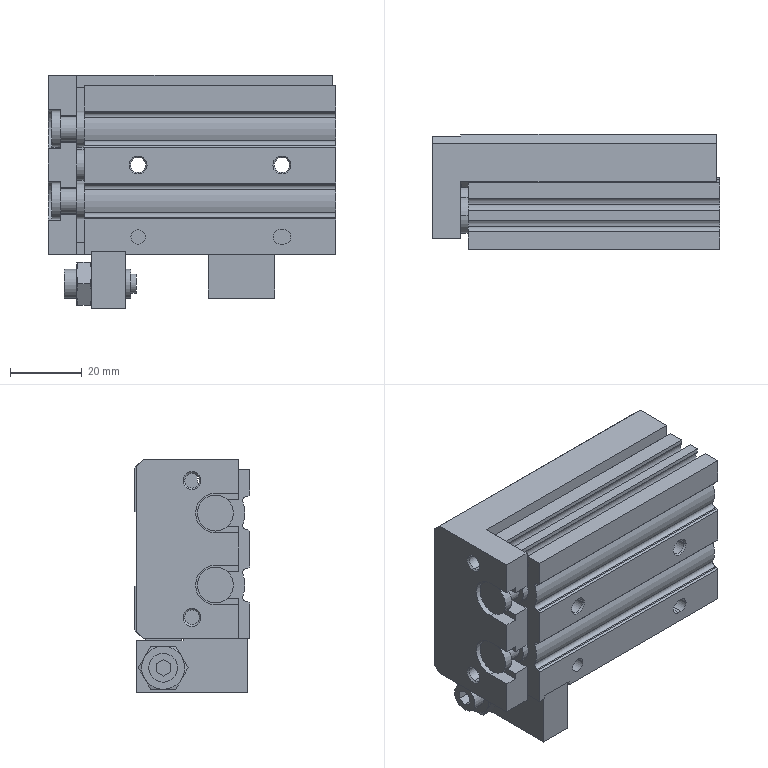Part | SolidWorks | features AEMSimFeature 1 | 6 solids | 432 faces | box 80 x 32 x 65 mm | volume 107710 mm3 | plane 228 | cylinder 140 | cone 64 | commonest cylinder face diameters 3.242 x24 4 x12 7.5 x10 4.134 x8 4.2 x8 6 x8